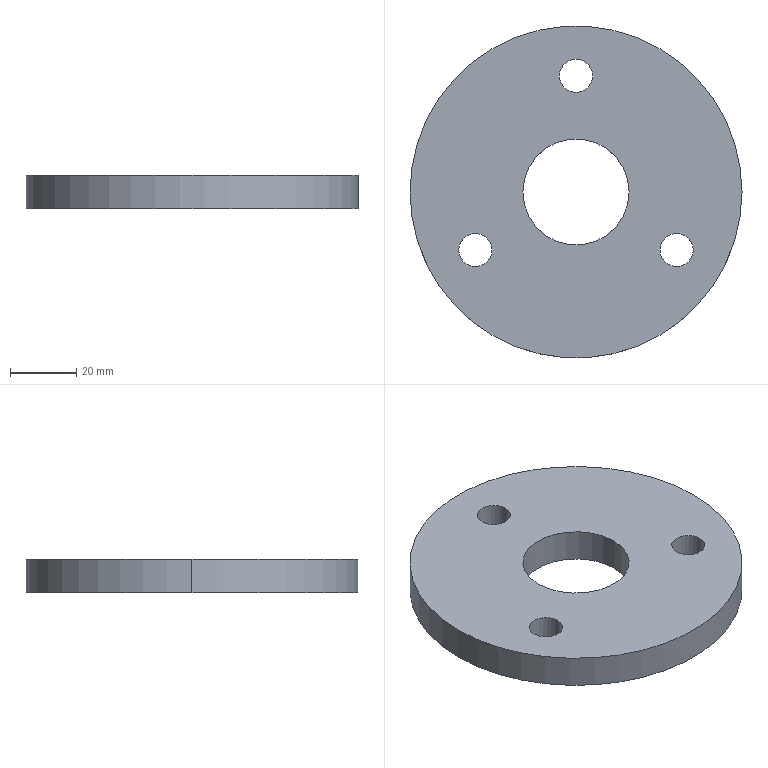Part | SolidWorks | features ICE 2, CirPattern 1, Extrusion 1 | 1 solid | 12 faces | box 100 x 100 x 10 mm | volume 68141 mm3 | cylinder 10 | plane 2 | commonest cylinder face diameters 10 x6 32 x2 100 x2
STEP:
#1=CARTESIAN_POINT('',(-16.,0.,0.));
#2=VERTEX_POINT('',#1);
#3=CARTESIAN_POINT('',(16.,0.,0.));
#4=VERTEX_POINT('',#3);
#5=CARTESIAN_POINT('',(0.,0.,0.));
#6=DIRECTION('',(0.,0.,1.));
#7=DIRECTION('',(1.,0.,0.));
#8=AXIS2_PLACEMENT_3D('',#5,#6,#7);
#9=CIRCLE('',#8,16.);
#10=EDGE_CURVE('',#2,#4,#9,.T.);
#11=ORIENTED_EDGE('',*,*,#10,.F.);
#12=CARTESIAN_POINT('',(-16.,0.,10.));
#13=VERTEX_POINT('',#12);
#14=CARTESIAN_POINT('',(-16.,0.,0.));
#15=DIRECTION('',(0.,0.,1.));
#16=VECTOR('',#15,1000.);
#17=LINE('',#14,#16);
#18=EDGE_CURVE('',#2,#13,#17,.T.);
#19=ORIENTED_EDGE('',*,*,#18,.T.);
#20=CARTESIAN_POINT('',(16.,0.,10.));
#21=VERTEX_POINT('',#20);
#22=CARTESIAN_POINT('',(0.,0.,10.));
#23=DIRECTION('',(0.,0.,1.));
#24=DIRECTION('',(1.,0.,0.));
#25=AXIS2_PLACEMENT_3D('',#22,#23,#24);
#26=CIRCLE('',#25,16.);
#27=EDGE_CURVE('',#13,#21,#26,.T.);
#28=ORIENTED_EDGE('',*,*,#27,.T.);
#29=CARTESIAN_POINT('',(16.,0.,0.));
#30=DIRECTION('',(0.,0.,1.));
#31=VECTOR('',#30,1000.);
#32=LINE('',#29,#31);
#33=EDGE_CURVE('',#4,#21,#32,.T.);
#34=ORIENTED_EDGE('',*,*,#33,.F.);
#35=EDGE_LOOP('',(#11,#19,#28,#34));
#36=FACE_OUTER_BOUND('',#35,.T.);
#37=CARTESIAN_POINT('',(0.,0.,0.));
#38=DIRECTION('',(0.,0.,1.));
#39=DIRECTION('',(1.,0.,0.));
#40=AXIS2_PLACEMENT_3D('',#37,#38,#39);
#41=CYLINDRICAL_SURFACE('',#40,16.);
#42=ADVANCED_FACE('',(#36),#41,.F.);
#43=CARTESIAN_POINT('',(-35.311,-17.5,0.));
#44=VERTEX_POINT('',#43);
#45=CARTESIAN_POINT('',(-25.311,-17.5,0.));
#46=VERTEX_POINT('',#45);
#47=CARTESIAN_POINT('',(-30.311,-17.5,0.));
#48=DIRECTION('',(0.,0.,1.));
#49=DIRECTION('',(-0.5,0.866,0.));
#50=AXIS2_PLACEMENT_3D('',#47,#48,#49);
#51=CIRCLE('',#50,5.);
#52=EDGE_CURVE('',#44,#46,#51,.T.);
#53=ORIENTED_EDGE('',*,*,#52,.F.);
#54=CARTESIAN_POINT('',(-35.311,-17.5,10.));
#55=VERTEX_POINT('',#54);
#56=CARTESIAN_POINT('',(-35.311,-17.5,0.));
#57=DIRECTION('',(0.,0.,1.));
#58=VECTOR('',#57,1000.);
#59=LINE('',#56,#58);
#60=EDGE_CURVE('',#44,#55,#59,.T.);
#61=ORIENTED_EDGE('',*,*,#60,.T.);
#62=CARTESIAN_POINT('',(-25.311,-17.5,10.));
#63=VERTEX_POINT('',#62);
#64=CARTESIAN_POINT('',(-30.311,-17.5,10.));
#65=DIRECTION('',(0.,0.,1.));
#66=DIRECTION('',(-0.5,0.866,0.));
#67=AXIS2_PLACEMENT_3D('',#64,#65,#66);
#68=CIRCLE('',#67,5.);
#69=EDGE_CURVE('',#55,#63,#68,.T.);
#70=ORIENTED_EDGE('',*,*,#69,.T.);
#71=CARTESIAN_POINT('',(-25.311,-17.5,0.));
#72=DIRECTION('',(0.,0.,1.));
#73=VECTOR('',#72,1000.);
#74=LINE('',#71,#73);
#75=EDGE_CURVE('',#46,#63,#74,.T.);
#76=ORIENTED_EDGE('',*,*,#75,.F.);
#77=EDGE_LOOP('',(#53,#61,#70,#76));
#78=FACE_OUTER_BOUND('',#77,.T.);
#79=CARTESIAN_POINT('',(-30.311,-17.5,0.));
#80=DIRECTION('',(0.,0.,1.));
#81=DIRECTION('',(1.,0.,0.));
#82=AXIS2_PLACEMENT_3D('',#79,#80,#81);
#83=CYLINDRICAL_SURFACE('',#82,5.);
#84=ADVANCED_FACE('',(#78),#83,.F.);
#85=CARTESIAN_POINT('',(25.311,-17.5,0.));
#86=VERTEX_POINT('',#85);
#87=CARTESIAN_POINT('',(35.311,-17.5,0.));
#88=VERTEX_POINT('',#87);
#89=CARTESIAN_POINT('',(30.311,-17.5,0.));
#90=DIRECTION('',(0.,0.,1.));
#91=DIRECTION('',(-0.5,-0.866,0.));
#92=AXIS2_PLACEMENT_3D('',#89,#90,#91);
#93=CIRCLE('',#92,5.);
#94=EDGE_CURVE('',#86,#88,#93,.T.);
#95=ORIENTED_EDGE('',*,*,#94,.F.);
#96=CARTESIAN_POINT('',(25.311,-17.5,10.));
#97=VERTEX_POINT('',#96);
#98=CARTESIAN_POINT('',(25.311,-17.5,0.));
#99=DIRECTION('',(0.,0.,1.));
#100=VECTOR('',#99,1000.);
#101=LINE('',#98,#100);
#102=EDGE_CURVE('',#86,#97,#101,.T.);
#103=ORIENTED_EDGE('',*,*,#102,.T.);
#104=CARTESIAN_POINT('',(35.311,-17.5,10.));
#105=VERTEX_POINT('',#104);
#106=CARTESIAN_POINT('',(30.311,-17.5,10.));
#107=DIRECTION('',(0.,0.,1.));
#108=DIRECTION('',(-0.5,-0.866,0.));
#109=AXIS2_PLACEMENT_3D('',#106,#107,#108);
#110=CIRCLE('',#109,5.);
#111=EDGE_CURVE('',#97,#105,#110,.T.);
#112=ORIENTED_EDGE('',*,*,#111,.T.);
#113=CARTESIAN_POINT('',(35.311,-17.5,0.));
#114=DIRECTION('',(0.,0.,1.));
#115=VECTOR('',#114,1000.);
#116=LINE('',#113,#115);
#117=EDGE_CURVE('',#88,#105,#116,.T.);
#118=ORIENTED_EDGE('',*,*,#117,.F.);
#119=EDGE_LOOP('',(#95,#103,#112,#118));
#120=FACE_OUTER_BOUND('',#119,.T.);
#121=CARTESIAN_POINT('',(30.311,-17.5,0.));
#122=DIRECTION('',(0.,0.,1.));
#123=DIRECTION('',(1.,0.,0.));
#124=AXIS2_PLACEMENT_3D('',#121,#122,#123);
#125=CYLINDRICAL_SURFACE('',#124,5.);
#126=ADVANCED_FACE('',(#120),#125,.F.);
#127=CARTESIAN_POINT('',(-5.,35.,0.));
#128=VERTEX_POINT('',#127);
#129=CARTESIAN_POINT('',(5.,35.,0.));
#130=VERTEX_POINT('',#129);
#131=CARTESIAN_POINT('',(0.,35.,0.));
#132=DIRECTION('',(0.,0.,1.));
#133=DIRECTION('',(1.,0.,0.));
#134=AXIS2_PLACEMENT_3D('',#131,#132,#133);
#135=CIRCLE('',#134,5.);
#136=EDGE_CURVE('',#128,#130,#135,.T.);
#137=ORIENTED_EDGE('',*,*,#136,.F.);
#138=CARTESIAN_POINT('',(-5.,35.,10.));
#139=VERTEX_POINT('',#138);
#140=CARTESIAN_POINT('',(-5.,35.,0.));
#141=DIRECTION('',(0.,0.,1.));
#142=VECTOR('',#141,1000.);
#143=LINE('',#140,#142);
#144=EDGE_CURVE('',#128,#139,#143,.T.);
#145=ORIENTED_EDGE('',*,*,#144,.T.);
#146=CARTESIAN_POINT('',(5.,35.,10.));
#147=VERTEX_POINT('',#146);
#148=CARTESIAN_POINT('',(0.,35.,10.));
#149=DIRECTION('',(0.,0.,1.));
#150=DIRECTION('',(1.,0.,0.));
#151=AXIS2_PLACEMENT_3D('',#148,#149,#150);
#152=CIRCLE('',#151,5.);
#153=EDGE_CURVE('',#139,#147,#152,.T.);
#154=ORIENTED_EDGE('',*,*,#153,.T.);
#155=CARTESIAN_POINT('',(5.,35.,0.));
#156=DIRECTION('',(0.,0.,1.));
#157=VECTOR('',#156,1000.);
#158=LINE('',#155,#157);
#159=EDGE_CURVE('',#130,#147,#158,.T.);
#160=ORIENTED_EDGE('',*,*,#159,.F.);
#161=EDGE_LOOP('',(#137,#145,#154,#160));
#162=FACE_OUTER_BOUND('',#161,.T.);
#163=CARTESIAN_POINT('',(0.,35.,0.));
#164=DIRECTION('',(0.,0.,1.));
#165=DIRECTION('',(1.,0.,0.));
#166=AXIS2_PLACEMENT_3D('',#163,#164,#165);
#167=CYLINDRICAL_SURFACE('',#166,5.);
#168=ADVANCED_FACE('',(#162),#167,.F.);
#169=CARTESIAN_POINT('',(50.,0.,10.));
#170=VERTEX_POINT('',#169);
#171=CARTESIAN_POINT('',(-50.,0.,10.));
#172=VERTEX_POINT('',#171);
#173=CARTESIAN_POINT('',(0.,0.,10.));
#174=DIRECTION('',(0.,0.,1.));
#175=DIRECTION('',(1.,0.,0.));
#176=AXIS2_PLACEMENT_3D('',#173,#174,#175);
#177=CIRCLE('',#176,50.);
#178=EDGE_CURVE('',#170,#172,#177,.T.);
#179=ORIENTED_EDGE('',*,*,#178,.F.);
#180=CARTESIAN_POINT('',(50.,0.,0.));
#181=VERTEX_POINT('',#180);
#182=CARTESIAN_POINT('',(50.,0.,10.));
#183=DIRECTION('',(0.,0.,-1.));
#184=VECTOR('',#183,1000.);
#185=LINE('',#182,#184);
#186=EDGE_CURVE('',#170,#181,#185,.T.);
#187=ORIENTED_EDGE('',*,*,#186,.T.);
#188=CARTESIAN_POINT('',(-50.,0.,0.));
#189=VERTEX_POINT('',#188);
#190=CARTESIAN_POINT('',(0.,0.,0.));
#191=DIRECTION('',(0.,0.,1.));
#192=DIRECTION('',(1.,0.,0.));
#193=AXIS2_PLACEMENT_3D('',#190,#191,#192);
#194=CIRCLE('',#193,50.);
#195=EDGE_CURVE('',#181,#189,#194,.T.);
#196=ORIENTED_EDGE('',*,*,#195,.T.);
#197=CARTESIAN_POINT('',(-50.,0.,10.));
#198=DIRECTION('',(0.,0.,-1.));
#199=VECTOR('',#198,1000.);
#200=LINE('',#197,#199);
#201=EDGE_CURVE('',#172,#189,#200,.T.);
#202=ORIENTED_EDGE('',*,*,#201,.F.);
#203=EDGE_LOOP('',(#179,#187,#196,#202));
#204=FACE_OUTER_BOUND('',#203,.T.);
#205=CARTESIAN_POINT('',(0.,0.,10.));
#206=DIRECTION('',(0.,0.,-1.));
#207=DIRECTION('',(-1.,0.,0.));
#208=AXIS2_PLACEMENT_3D('',#205,#206,#207);
#209=CYLINDRICAL_SURFACE('',#208,50.);
#210=ADVANCED_FACE('',(#204),#209,.T.);
#211=ORIENTED_EDGE('',*,*,#186,.F.);
#212=CARTESIAN_POINT('',(0.,0.,10.));
#213=DIRECTION('',(0.,0.,1.));
#214=DIRECTION('',(1.,0.,0.));
#215=AXIS2_PLACEMENT_3D('',#212,#213,#214);
#216=CIRCLE('',#215,50.);
#217=EDGE_CURVE('',#172,#170,#216,.T.);
#218=ORIENTED_EDGE('',*,*,#217,.F.);
#219=ORIENTED_EDGE('',*,*,#201,.T.);
#220=CARTESIAN_POINT('',(0.,0.,0.));
#221=DIRECTION('',(0.,0.,1.));
#222=DIRECTION('',(1.,0.,0.));
#223=AXIS2_PLACEMENT_3D('',#220,#221,#222);
#224=CIRCLE('',#223,50.);
#225=EDGE_CURVE('',#189,#181,#224,.T.);
#226=ORIENTED_EDGE('',*,*,#225,.T.);
#227=EDGE_LOOP('',(#211,#218,#219,#226));
#228=FACE_OUTER_BOUND('',#227,.T.);
#229=CARTESIAN_POINT('',(0.,0.,10.));
#230=DIRECTION('',(0.,0.,-1.));
#231=DIRECTION('',(-1.,0.,0.));
#232=AXIS2_PLACEMENT_3D('',#229,#230,#231);
#233=CYLINDRICAL_SURFACE('',#232,50.);
#234=ADVANCED_FACE('',(#228),#233,.T.);
#235=CARTESIAN_POINT('',(0.,0.,10.));
#236=DIRECTION('',(0.,0.,1.));
#237=DIRECTION('',(1.,0.,0.));
#238=AXIS2_PLACEMENT_3D('',#235,#236,#237);
#239=CIRCLE('',#238,16.);
#240=EDGE_CURVE('',#21,#13,#239,.T.);
#241=ORIENTED_EDGE('',*,*,#240,.F.);
#242=ORIENTED_EDGE('',*,*,#27,.F.);
#243=EDGE_LOOP('',(#241,#242));
#244=FACE_BOUND('',#243,.T.);
#245=CARTESIAN_POINT('',(-30.311,-17.5,10.));
#246=DIRECTION('',(0.,0.,1.));
#247=DIRECTION('',(-0.5,0.866,0.));
#248=AXIS2_PLACEMENT_3D('',#245,#246,#247);
#249=CIRCLE('',#248,5.);
#250=EDGE_CURVE('',#63,#55,#249,.T.);
#251=ORIENTED_EDGE('',*,*,#250,.F.);
#252=ORIENTED_EDGE('',*,*,#69,.F.);
#253=EDGE_LOOP('',(#251,#252));
#254=FACE_BOUND('',#253,.T.);
#255=CARTESIAN_POINT('',(30.311,-17.5,10.));
#256=DIRECTION('',(0.,0.,1.));
#257=DIRECTION('',(-0.5,-0.866,0.));
#258=AXIS2_PLACEMENT_3D('',#255,#256,#257);
#259=CIRCLE('',#258,5.);
#260=EDGE_CURVE('',#105,#97,#259,.T.);
#261=ORIENTED_EDGE('',*,*,#260,.F.);
#262=ORIENTED_EDGE('',*,*,#111,.F.);
#263=EDGE_LOOP('',(#261,#262));
#264=FACE_BOUND('',#263,.T.);
#265=CARTESIAN_POINT('',(0.,35.,10.));
#266=DIRECTION('',(0.,0.,1.));
#267=DIRECTION('',(1.,0.,0.));
#268=AXIS2_PLACEMENT_3D('',#265,#266,#267);
#269=CIRCLE('',#268,5.);
#270=EDGE_CURVE('',#147,#139,#269,.T.);
#271=ORIENTED_EDGE('',*,*,#270,.F.);
#272=ORIENTED_EDGE('',*,*,#153,.F.);
#273=EDGE_LOOP('',(#271,#272));
#274=FACE_BOUND('',#273,.T.);
#275=ORIENTED_EDGE('',*,*,#217,.T.);
#276=ORIENTED_EDGE('',*,*,#178,.T.);
#277=EDGE_LOOP('',(#275,#276));
#278=FACE_OUTER_BOUND('',#277,.T.);
#279=CARTESIAN_POINT('',(0.,0.,10.));
#280=DIRECTION('',(0.,0.,1.));
#281=DIRECTION('',(1.,0.,0.));
#282=AXIS2_PLACEMENT_3D('',#279,#280,#281);
#283=PLANE('',#282);
#284=ADVANCED_FACE('',(#244,#254,#264,#274,#278),#283,.T.);
#285=CARTESIAN_POINT('',(0.,0.,0.));
#286=DIRECTION('',(0.,0.,1.));
#287=DIRECTION('',(1.,0.,0.));
#288=AXIS2_PLACEMENT_3D('',#285,#286,#287);
#289=CIRCLE('',#288,16.);
#290=EDGE_CURVE('',#4,#2,#289,.T.);
#291=ORIENTED_EDGE('',*,*,#290,.T.);
#292=ORIENTED_EDGE('',*,*,#10,.T.);
#293=EDGE_LOOP('',(#291,#292));
#294=FACE_BOUND('',#293,.T.);
#295=CARTESIAN_POINT('',(-30.311,-17.5,0.));
#296=DIRECTION('',(0.,0.,1.));
#297=DIRECTION('',(-0.5,0.866,0.));
#298=AXIS2_PLACEMENT_3D('',#295,#296,#297);
#299=CIRCLE('',#298,5.);
#300=EDGE_CURVE('',#46,#44,#299,.T.);
#301=ORIENTED_EDGE('',*,*,#300,.T.);
#302=ORIENTED_EDGE('',*,*,#52,.T.);
#303=EDGE_LOOP('',(#301,#302));
#304=FACE_BOUND('',#303,.T.);
#305=CARTESIAN_POINT('',(30.311,-17.5,0.));
#306=DIRECTION('',(0.,0.,1.));
#307=DIRECTION('',(-0.5,-0.866,0.));
#308=AXIS2_PLACEMENT_3D('',#305,#306,#307);
#309=CIRCLE('',#308,5.);
#310=EDGE_CURVE('',#88,#86,#309,.T.);
#311=ORIENTED_EDGE('',*,*,#310,.T.);
#312=ORIENTED_EDGE('',*,*,#94,.T.);
#313=EDGE_LOOP('',(#311,#312));
#314=FACE_BOUND('',#313,.T.);
#315=CARTESIAN_POINT('',(0.,35.,0.));
#316=DIRECTION('',(0.,0.,1.));
#317=DIRECTION('',(1.,0.,0.));
#318=AXIS2_PLACEMENT_3D('',#315,#316,#317);
#319=CIRCLE('',#318,5.);
#320=EDGE_CURVE('',#130,#128,#319,.T.);
#321=ORIENTED_EDGE('',*,*,#320,.T.);
#322=ORIENTED_EDGE('',*,*,#136,.T.);
#323=EDGE_LOOP('',(#321,#322));
#324=FACE_BOUND('',#323,.T.);
#325=ORIENTED_EDGE('',*,*,#225,.F.);
#326=ORIENTED_EDGE('',*,*,#195,.F.);
#327=EDGE_LOOP('',(#325,#326));
#328=FACE_OUTER_BOUND('',#327,.T.);
#329=CARTESIAN_POINT('',(0.,0.,0.));
#330=DIRECTION('',(0.,0.,1.));
#331=DIRECTION('',(1.,0.,0.));
#332=AXIS2_PLACEMENT_3D('',#329,#330,#331);
#333=PLANE('',#332);
#334=ADVANCED_FACE('',(#294,#304,#314,#324,#328),#333,.F.);
#335=ORIENTED_EDGE('',*,*,#144,.F.);
#336=ORIENTED_EDGE('',*,*,#320,.F.);
#337=ORIENTED_EDGE('',*,*,#159,.T.);
#338=ORIENTED_EDGE('',*,*,#270,.T.);
#339=EDGE_LOOP('',(#335,#336,#337,#338));
#340=FACE_OUTER_BOUND('',#339,.T.);
#341=CARTESIAN_POINT('',(0.,35.,0.));
#342=DIRECTION('',(0.,0.,1.));
#343=DIRECTION('',(1.,0.,0.));
#344=AXIS2_PLACEMENT_3D('',#341,#342,#343);
#345=CYLINDRICAL_SURFACE('',#344,5.);
#346=ADVANCED_FACE('',(#340),#345,.F.);
#347=ORIENTED_EDGE('',*,*,#102,.F.);
#348=ORIENTED_EDGE('',*,*,#310,.F.);
#349=ORIENTED_EDGE('',*,*,#117,.T.);
#350=ORIENTED_EDGE('',*,*,#260,.T.);
#351=EDGE_LOOP('',(#347,#348,#349,#350));
#352=FACE_OUTER_BOUND('',#351,.T.);
#353=CARTESIAN_POINT('',(30.311,-17.5,0.));
#354=DIRECTION('',(0.,0.,1.));
#355=DIRECTION('',(1.,0.,0.));
#356=AXIS2_PLACEMENT_3D('',#353,#354,#355);
#357=CYLINDRICAL_SURFACE('',#356,5.);
#358=ADVANCED_FACE('',(#352),#357,.F.);
#359=ORIENTED_EDGE('',*,*,#60,.F.);
#360=ORIENTED_EDGE('',*,*,#300,.F.);
#361=ORIENTED_EDGE('',*,*,#75,.T.);
#362=ORIENTED_EDGE('',*,*,#250,.T.);
#363=EDGE_LOOP('',(#359,#360,#361,#362));
#364=FACE_OUTER_BOUND('',#363,.T.);
#365=CARTESIAN_POINT('',(-30.311,-17.5,0.));
#366=DIRECTION('',(0.,0.,1.));
#367=DIRECTION('',(1.,0.,0.));
#368=AXIS2_PLACEMENT_3D('',#365,#366,#367);
#369=CYLINDRICAL_SURFACE('',#368,5.);
#370=ADVANCED_FACE('',(#364),#369,.F.);
#371=ORIENTED_EDGE('',*,*,#18,.F.);
#372=ORIENTED_EDGE('',*,*,#290,.F.);
#373=ORIENTED_EDGE('',*,*,#33,.T.);
#374=ORIENTED_EDGE('',*,*,#240,.T.);
#375=EDGE_LOOP('',(#371,#372,#373,#374));
#376=FACE_OUTER_BOUND('',#375,.T.);
#377=CARTESIAN_POINT('',(0.,0.,0.));
#378=DIRECTION('',(0.,0.,1.));
#379=DIRECTION('',(1.,0.,0.));
#380=AXIS2_PLACEMENT_3D('',#377,#378,#379);
#381=CYLINDRICAL_SURFACE('',#380,16.);
#382=ADVANCED_FACE('',(#376),#381,.F.);
#383=CLOSED_SHELL('',(#42,#84,#126,#168,#210,#234,#284,#334,#346,#358,#370,#382));
#384=MANIFOLD_SOLID_BREP('',#383);
#385=CARTESIAN_POINT('',(0.,0.,0.));
#386=DIRECTION('',(0.,0.,1.));
#387=DIRECTION('',(1.,0.,0.));
#388=AXIS2_PLACEMENT_3D('',#385,#386,#387);
#389=(LENGTH_UNIT()NAMED_UNIT(*)SI_UNIT(.MILLI.,.METRE.));
#390=UNCERTAINTY_MEASURE_WITH_UNIT(LENGTH_MEASURE(0.00001),#389,'','');
#391=(NAMED_UNIT(*)PLANE_ANGLE_UNIT()SI_UNIT($,.RADIAN.));
#392=(NAMED_UNIT(*)SI_UNIT($,.STERADIAN.)SOLID_ANGLE_UNIT());
#393=(GEOMETRIC_REPRESENTATION_CONTEXT(3)GLOBAL_UNCERTAINTY_ASSIGNED_CONTEXT((#390))GLOBAL_UNIT_ASSIGNED_CONTEXT((#389,#391,#392))REPRESENTATION_CONTEXT('',''));
#394=ADVANCED_BREP_SHAPE_REPRESENTATION('',(#384,#388),#393);